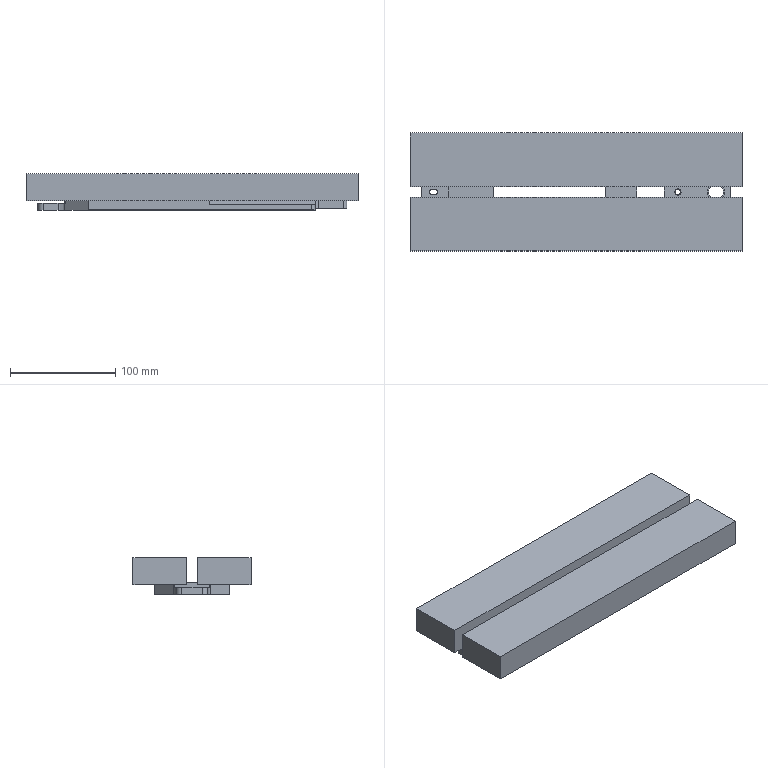NC program | NX | posted with a generic post | part box 315 x 112 x 34.85 mm
Lines 3199 to 4522 of 11462:
(ADAPTIVE_MILLING_COPY , TOOL : D4开粗)
N6390 T03 M6
N6392 G53
N6394 G17 G0 G90 X121.904 Y19.81 S6500 M3
N6396 G43 Z20. H3
N6398 Z-10.
N6400 G94 G1 X121.804 Y19.803 Z-10.625 F2000.
N6402 X121.705 Y19.797 Z-10.872
N6404 X121.605 Y19.79 Z-11.054
N6406 X121.505 Y19.783 Z-11.2
N6408 X121.405 Y19.776 Z-11.323
N6410 X121.306 Y19.769 Z-11.428
N6412 X121.206 Y19.762 Z-11.52
N6414 X121.106 Y19.755 Z-11.6
N6416 X121.006 Y19.748 Z-11.67
N6418 X120.907 Y19.741 Z-11.732
N6420 X120.807 Y19.734 Z-11.786
N6422 X120.707 Y19.727 Z-11.833
N6424 X120.607 Y19.72 Z-11.874
N6426 X120.507 Y19.713 Z-11.908
N6428 X120.408 Y19.706 Z-11.936
N6430 X120.308 Y19.699 Z-11.96
N6432 X120.208 Y19.692 Z-11.977
N6434 X120.108 Y19.685 Z-11.99
N6436 X120.009 Y19.678 Z-11.997
N6438 X119.909 Y19.671 Z-12.
N6440 X119.565 Y19.651
N6442 X119.222 Y19.614
N6444 G3 X118.932 Y19.226 R0.405
N6446 X119.957 Y16.307 R3.97
N6448 X122.288 Y14.7 R5.019
N6450 G1 X123.6
N6452 G2 X121.918 Y14.735 R12.158
N6454 X119.43 Y16.653 R4.439
N6456 X118.934 Y17.688 R3.914
N6458 G1 X118.933 Y18.626
N6460 G3 X118.965 Y17.166 R10.215
N6462 X121.068 Y14.709 R3.865
N6464 G1 X122.177 Y14.7
N6466 X120.959 Y14.713
N6468 G2 X119.174 Y16.174 R3.119
N6470 X118.936 Y16.705 R2.049
N6472 G1 X118.935 Y17.417
N6474 G3 X118.981 Y16.226 R5.673
N6476 X120.256 Y14.709 R2.419
N6478 G1 X121.068 Y14.7
N6480 G2 X120.115 Y14.725 R4.858
N6482 X118.937 Y15.953 R1.926
N6484 G1 X118.936 Y16.516
N6486 G3 X118.983 Y15.549 R3.764
N6488 X119.671 Y14.716 R1.364
N6490 G1 X120.245 Y14.7
N6492 G2 X119.567 Y14.73 R2.419
N6494 X118.937 Y15.773 R0.951
N6496 G3 X118.964 Y15.262 R4.171
N6498 X119.494 Y14.731 R1.08
N6500 G1 X119.676 Y14.702
N6502 G3 X120.106 Y15.099 R0.404
N6504 G1 X120.115 Y15.688
N6506 X120.116 Y15.788 Z-11.997
N6508 X120.118 Y15.888 Z-11.99
N6510 X120.119 Y15.988 Z-11.977
N6512 X120.121 Y16.088 Z-11.96
N6514 X120.122 Y16.188 Z-11.936
N6516 X120.124 Y16.288 Z-11.908
N6518 X120.126 Y16.388 Z-11.874
N6520 X120.127 Y16.488 Z-11.833
N6522 X120.129 Y16.588 Z-11.786
N6524 X120.13 Y16.688 Z-11.732
N6526 X120.132 Y16.788 Z-11.67
N6528 X120.133 Y16.888 Z-11.6
N6530 X120.135 Y16.988 Z-11.52
N6532 X120.136 Y17.088 Z-11.428
N6534 X120.138 Y17.188 Z-11.323
N6536 X120.139 Y17.288 Z-11.2
N6538 X120.141 Y17.388 Z-11.054
N6540 X120.142 Y17.488 Z-10.872
N6542 X120.144 Y17.588 Z-10.625
N6544 X120.145 Y17.688 Z-10.
N6546 G0 Z20.
N6548 X123.964 Y-17.678
N6550 Z-10.
N6552 G1 X123.962 Y-17.578 Z-10.625
N6554 X123.96 Y-17.478 Z-10.872
N6556 X123.959 Y-17.378 Z-11.054
N6558 X123.957 Y-17.278 Z-11.2
N6560 X123.955 Y-17.178 Z-11.323
N6562 X123.953 Y-17.078 Z-11.428
N6564 X123.952 Y-16.978 Z-11.52
N6566 X123.95 Y-16.878 Z-11.6
N6568 X123.948 Y-16.778 Z-11.67
N6570 X123.947 Y-16.678 Z-11.732
N6572 X123.945 Y-16.578 Z-11.786
N6574 X123.943 Y-16.478 Z-11.833
N6576 X123.941 Y-16.378 Z-11.874
N6578 X123.94 Y-16.278 Z-11.908
N6580 X123.938 Y-16.178 Z-11.936
N6582 X123.936 Y-16.078 Z-11.96
N6584 X123.935 Y-15.978 Z-11.977
N6586 X123.933 Y-15.878 Z-11.99
N6588 X123.931 Y-15.778 Z-11.997
N6590 X123.929 Y-15.678 Z-12.
N6592 X123.919 Y-15.097
N6594 G3 X123.515 Y-14.7 R0.404
N6596 X120.433 Y-15.812 R4.064
N6598 X118.911 Y-18.098 R5.039
N6600 G1 Y-19.336
N6602 G2 X118.947 Y-17.724 R11.256
N6604 X121.099 Y-15.067 R4.557
N6606 X121.932 Y-14.7 R3.985
N6608 G1 X122.832
N6610 G3 X121.442 Y-14.721 R15.425
N6612 X119.137 Y-16.454 R3.876
N6614 X118.911 Y-16.925 R1.387
N6616 G1 Y-18.013
N6618 X118.924 Y-16.757
N6620 G2 X120.344 Y-14.977 R3.165
N6622 X120.94 Y-14.7 R2.17
N6624 G1 X121.615
N6626 G3 X120.446 Y-14.749 R5.1
N6628 X118.928 Y-16.015 R2.666
N6630 G1 X118.911 Y-16.854
N6632 G2 X118.93 Y-15.934 R14.426
N6634 X120.192 Y-14.7 R1.931
N6636 G1 X120.717
N6638 G3 X119.73 Y-14.764 R3.043
N6640 X118.921 Y-15.476 R1.314
N6642 G1 X118.911 Y-16.03
N6644 G2 X118.958 Y-15.307 R2.219
N6646 X120.024 Y-14.7 R0.974
N6648 G3 X119.37 Y-14.781 R1.316
N6650 X118.927 Y-15.393 R1.202
N6652 X119.331 Y-15.862 R0.404
N6654 G1 X119.898 Y-15.854
N6656 X119.998 Y-15.853 Z-11.997
N6658 X120.098 Y-15.852 Z-11.99
N6660 X120.198 Y-15.851 Z-11.977
N6662 X120.298 Y-15.849 Z-11.96
N6664 X120.398 Y-15.848 Z-11.936
N6666 X120.498 Y-15.847 Z-11.908
N6668 X120.598 Y-15.845 Z-11.874
N6670 X120.698 Y-15.844 Z-11.833
N6672 X120.798 Y-15.843 Z-11.786
N6674 X120.898 Y-15.842 Z-11.732
N6676 X120.998 Y-15.84 Z-11.67
N6678 X121.098 Y-15.839 Z-11.6
N6680 X121.198 Y-15.838 Z-11.52
N6682 X121.298 Y-15.837 Z-11.428
N6684 X121.398 Y-15.835 Z-11.323
N6686 X121.498 Y-15.834 Z-11.2
N6688 X121.598 Y-15.833 Z-11.054
N6690 X121.698 Y-15.832 Z-10.872
N6692 X121.798 Y-15.83 Z-10.625
N6694 X121.898 Y-15.829 Z-10.
N6696 G0 Z20.
N6698 X134.278 Y0.889
N6700 Z2.
N6702 G3 X134.278 Y0.889 Z1.803 I-1.564 J-0.891
N6704 X134.278 Y0.889 Z1.605 I-1.564 J-0.891
N6706 X134.278 Y0.889 Z1.408 I-1.564 J-0.891
N6708 X134.278 Y0.889 Z1.21 I-1.564 J-0.891
N6710 X134.278 Y0.889 Z1.013 I-1.564 J-0.891
N6712 X134.278 Y0.889 Z0.816 I-1.564 J-0.891
N6714 X134.278 Y0.889 Z0.618 I-1.564 J-0.891
N6716 X134.278 Y0.889 Z0.421 I-1.564 J-0.891
N6718 X134.278 Y0.889 Z0.223 I-1.564 J-0.891
N6720 X134.278 Y0.889 Z0.026 I-1.564 J-0.891
N6722 X134.278 Y0.889 Z-0.172 I-1.564 J-0.891
N6724 X134.278 Y0.889 Z-0.369 I-1.564 J-0.891
N6726 X134.278 Y0.889 Z-0.566 I-1.564 J-0.891
N6728 X134.278 Y0.889 Z-0.764 I-1.564 J-0.891
N6730 X134.278 Y0.889 Z-0.961 I-1.564 J-0.891
N6732 X134.278 Y0.889 Z-1.159 I-1.564 J-0.891
N6734 X134.278 Y0.889 Z-1.356 I-1.564 J-0.891
N6736 X134.278 Y0.889 Z-1.553 I-1.564 J-0.891
N6738 X134.278 Y0.889 Z-1.751 I-1.564 J-0.891
N6740 X134.278 Y0.889 Z-1.948 I-1.564 J-0.891
N6742 X134.278 Y0.889 Z-2.146 I-1.564 J-0.891
N6744 X134.278 Y0.889 Z-2.343 I-1.564 J-0.891
N6746 X134.278 Y0.889 Z-2.54 I-1.564 J-0.891
N6748 X134.278 Y0.889 Z-2.738 I-1.564 J-0.891
N6750 X134.278 Y0.889 Z-2.935 I-1.564 J-0.891
N6752 X134.278 Y0.889 Z-3.133 I-1.564 J-0.891
N6754 X134.278 Y0.889 Z-3.33 I-1.564 J-0.891
N6756 X134.278 Y0.889 Z-3.528 I-1.564 J-0.891
N6758 X134.278 Y0.889 Z-3.725 I-1.564 J-0.891
N6760 X134.278 Y0.889 Z-3.922 I-1.564 J-0.891
N6762 X134.278 Y0.889 Z-4.12 I-1.564 J-0.891
N6764 X134.278 Y0.889 Z-4.317 I-1.564 J-0.891
N6766 X134.278 Y0.889 Z-4.515 I-1.564 J-0.891
N6768 X134.278 Y0.889 Z-4.712 I-1.564 J-0.891
N6770 X134.278 Y0.889 Z-4.909 I-1.564 J-0.891
N6772 X134.278 Y0.889 Z-5.107 I-1.564 J-0.891
N6774 X134.278 Y0.889 Z-5.304 I-1.564 J-0.891
N6776 X134.278 Y0.889 Z-5.502 I-1.564 J-0.891
N6778 X134.278 Y0.889 Z-5.699 I-1.564 J-0.891
N6780 X134.278 Y0.889 Z-5.896 I-1.564 J-0.891
N6782 X134.278 Y0.889 Z-6.094 I-1.564 J-0.891
N6784 X134.278 Y0.889 Z-6.291 I-1.564 J-0.891
N6786 X134.278 Y0.889 Z-6.489 I-1.564 J-0.891
N6788 X134.278 Y0.889 Z-6.686 I-1.564 J-0.891
N6790 X134.278 Y0.889 Z-6.884 I-1.564 J-0.891
N6792 X134.278 Y0.889 Z-7.081 I-1.564 J-0.891
N6794 X134.278 Y0.889 Z-7.278 I-1.564 J-0.891
N6796 X134.278 Y0.889 Z-7.476 I-1.564 J-0.891
N6798 X134.278 Y0.889 Z-7.673 I-1.564 J-0.891
N6800 X134.278 Y0.889 Z-7.871 I-1.564 J-0.891
N6802 X134.278 Y0.889 Z-8.068 I-1.564 J-0.891
N6804 X134.278 Y0.889 Z-8.265 I-1.564 J-0.891
N6806 X134.278 Y0.889 Z-8.463 I-1.564 J-0.891
N6808 X134.278 Y0.889 Z-8.66 I-1.564 J-0.891
N6810 X134.278 Y0.889 Z-8.858 I-1.564 J-0.891
N6812 X134.278 Y0.889 Z-9.055 I-1.564 J-0.891
N6814 X134.278 Y0.889 Z-9.252 I-1.564 J-0.891
N6816 X134.278 Y0.889 Z-9.45 I-1.564 J-0.891
N6818 X134.278 Y0.889 Z-9.647 I-1.564 J-0.891
N6820 X134.278 Y0.889 Z-9.845 I-1.564 J-0.891
N6822 X134.278 Y0.889 Z-10.042 I-1.564 J-0.891
N6824 X134.278 Y0.889 Z-10.24 I-1.564 J-0.891
N6826 X134.278 Y0.889 Z-10.437 I-1.564 J-0.891
N6828 X134.278 Y0.889 Z-10.634 I-1.564 J-0.891
N6830 X134.278 Y0.889 Z-10.832 I-1.564 J-0.891
N6832 X134.278 Y0.889 Z-11.029 I-1.564 J-0.891
N6834 X134.278 Y0.889 Z-11.227 I-1.564 J-0.891
N6836 X134.278 Y0.889 Z-11.424 I-1.564 J-0.891
N6838 X134.278 Y0.889 Z-11.621 I-1.564 J-0.891
N6840 X134.278 Y0.889 Z-11.819 I-1.564 J-0.891
N6842 X134.513 Y-0.002 Z-12. R-1.8
N6844 X133.169 Y-1.769 R-1.812
N6846 X134.378 Y1.134 R1.985
N6848 X131.316 Y-1.517 R-2.04
N6850 X134.785 Y-0.555 R2.149
N6852 X131.6 Y2.013 R2.19
N6854 X134.178 Y-1.829 R-2.321
N6856 X131.742 Y2.378 R2.448
N6858 X134.157 Y-2.179 R-2.59
N6860 X131.562 Y2.607 R2.728
N6862 X134.288 Y-2.437 R-2.875
N6864 X131.354 Y2.834 R3.02
N6866 X134.271 Y-2.792 R-3.17
N6868 X131.293 Y3.141 R3.321
N6870 X134.269 Y-3.141 R-3.476
N6872 X131.393 Y3.522 R3.632
N6874 X129.192 Y-1.367 R3.791
N6876 X134.1 Y-3.561 R3.791
N6878 X131.462 Y3.888 R3.952
N6880 X134.377 Y-3.804 R-4.117
N6882 X131.257 Y4.171 R4.284
N6884 X134.314 Y-4.192 R-4.452
N6886 X131.411 Y4.575 R4.621
N6888 X128.891 Y2.852 R4.753
N6890 X129.877 Y-3.871 R4.764
N6892 X132.631 Y-4.795 R5.129
N6894 X136.255 Y-3.234 R4.972
N6896 X135.347 Y4.007 R4.816
N6898 X133.403 Y4.748 R5.586
N6900 X130.734 Y4.369 R5.227
N6902 X129.688 Y3.725 R7.287
N6904 G1 X128.929 Y2.948
N6906 G3 X128.027 Y1.029 R5.459
N6908 X127.928 Y-0.178 R5.861
N6910 X128.347 Y-1.982 R4.669
N6912 X129.877 Y-3.871 R4.678
N6914 G1 X130.771 Y-4.383
N6916 G3 X131.297 Y-4.089 R0.404
N6918 G1 X131.415 Y-3.565
N6920 X131.437 Y-3.467 Z-11.997
N6922 X131.459 Y-3.37 Z-11.99
N6924 X131.481 Y-3.272 Z-11.977
N6926 X131.503 Y-3.175 Z-11.96
N6928 X131.525 Y-3.077 Z-11.936
N6930 X131.547 Y-2.98 Z-11.908
N6932 X131.569 Y-2.882 Z-11.874
N6934 X131.591 Y-2.785 Z-11.833
N6936 X131.613 Y-2.687 Z-11.786
N6938 X131.635 Y-2.59 Z-11.732
N6940 X131.657 Y-2.492 Z-11.67
N6942 X131.679 Y-2.394 Z-11.6
N6944 X131.701 Y-2.297 Z-11.52
N6946 X131.723 Y-2.199 Z-11.428
N6948 X131.745 Y-2.102 Z-11.323
N6950 X131.767 Y-2.004 Z-11.2
N6952 X131.789 Y-1.907 Z-11.054
N6954 X131.811 Y-1.809 Z-10.872
N6956 X131.833 Y-1.712 Z-10.625
N6958 X131.855 Y-1.614 Z-10.
N6960 G0 Z20.
N6962 X130.749 Y3.453
N6964 Z-1.
N6966 G1 X130.686 Y3.376 Z-1.625
N6968 X130.622 Y3.298 Z-1.872
N6970 X130.559 Y3.221 Z-2.054
N6972 X130.495 Y3.144 Z-2.2
N6974 X130.432 Y3.066 Z-2.323
N6976 X130.368 Y2.989 Z-2.428
N6978 X130.305 Y2.912 Z-2.52
N6980 X130.241 Y2.835 Z-2.6
N6982 X130.178 Y2.757 Z-2.67
N6984 X130.114 Y2.68 Z-2.732
N6986 X130.051 Y2.603 Z-2.786
N6988 X129.987 Y2.526 Z-2.833
N6990 X129.924 Y2.448 Z-2.874
N6992 X129.86 Y2.371 Z-2.908
N6994 X129.797 Y2.294 Z-2.936
N6996 X129.733 Y2.217 Z-2.96
N6998 X129.67 Y2.139 Z-2.977
N7000 X129.606 Y2.062 Z-2.99
N7002 X129.543 Y1.985 Z-2.997
N7004 X129.479 Y1.908 Z-3.
N7006 X127.934 Y0.016
N7008 G3 X127.828 Y-1.414 R2.078
N7010 X131.848 Y-5.074 R4.902
N7012 X127.68 Y1.115 R-5.151
N7014 X127.732 Y-2.277 R4.916
N7016 X135.519 Y-4.758 R5.442
N7018 X127.427 Y1.649 R-5.528
N7020 X127.808 Y-3.225 R5.441
N7022 X138.044 Y2.534 R5.885
N7024 X127.193 Y2.139 R5.921
N7026 X126.664 Y-0.024 R6.313
N7028 X127.104 Y-2.263 R6.904
N7030 X128.26 Y-4.094 R6.989
N7032 X130.91 Y-5.774 R6.428
N7034 X133.23 Y-6.024 R7.001
N7036 X134.632 Y-5.734 R9.787
N7038 X137.27 Y-3.971 R6.477
N7040 X138.699 Y-0.84 R6.338
N7042 X138.369 Y2.133 R6.079
N7044 X136.469 Y4.736 R6.48
N7046 X134.312 Y5.831 R6.722
N7048 G1 X133.152 Y6.03
N7050 G3 X130.788 Y5.735 R6.94
N7052 X128.122 Y3.939 R6.486
N7054 X126.755 Y1.049 R6.445
N7056 G1 X126.693 Y0.377
N7058 G3 X127.185 Y-0.054 R0.404
N7060 G1 X127.648 Y0.05
N7062 X127.745 Y0.072 Z-2.997
N7064 X127.843 Y0.095 Z-2.99
N7066 X127.94 Y0.117 Z-2.977
N7068 X128.038 Y0.139 Z-2.96
N7070 X128.135 Y0.161 Z-2.936
N7072 X128.233 Y0.183 Z-2.908
N7074 X128.33 Y0.205 Z-2.874
N7076 X128.428 Y0.227 Z-2.833
N7078 X128.525 Y0.249 Z-2.786
N7080 X128.623 Y0.271 Z-2.732
N7082 X128.721 Y0.293 Z-2.67
N7084 X128.818 Y0.315 Z-2.6
N7086 X128.916 Y0.337 Z-2.52
N7088 X129.013 Y0.359 Z-2.428
N7090 X129.111 Y0.381 Z-2.323
N7092 X129.208 Y0.403 Z-2.2
N7094 X129.306 Y0.425 Z-2.054
N7096 X129.403 Y0.448 Z-1.872
N7098 X129.501 Y0.47 Z-1.625
N7100 X129.598 Y0.492 Z-1.
N7102 G0 Z20.
N7104 X64.758 Y11.336
N7106 Z-3.399
N7108 G1 X64.745 Y11.435 Z-4.024
N7110 X64.732 Y11.535 Z-4.271
N7112 X64.719 Y11.634 Z-4.453
N7114 X64.706 Y11.733 Z-4.599
N7116 X64.693 Y11.832 Z-4.722
N7118 X64.68 Y11.931 Z-4.827
N7120 X64.667 Y12.03 Z-4.919
N7122 X64.653 Y12.13 Z-4.999
N7124 X64.64 Y12.229 Z-5.069
N7126 X64.627 Y12.328 Z-5.131
N7128 X64.614 Y12.427 Z-5.185
N7130 X64.601 Y12.526 Z-5.232
N7132 X64.588 Y12.625 Z-5.273
N7134 X64.575 Y12.724 Z-5.307
N7136 X64.562 Y12.824 Z-5.335
N7138 X64.549 Y12.923 Z-5.359
N7140 X64.536 Y13.022 Z-5.376
N7142 X64.523 Y13.121 Z-5.389
N7144 X64.51 Y13.22 Z-5.396
N7146 X64.497 Y13.319 Z-5.399
N7148 X64.414 Y13.949
N7150 G3 X64.014 Y14.3 R0.405
N7152 X61.361 Y13.372 R3.686
N7154 X59.763 Y11.186 R5.239
N7156 G1 X59.76 Y9.995
N7158 G2 X59.786 Y11.45 R11.987
N7160 X61.618 Y13.825 R4.291
N7162 X62.599 Y14.3 R3.662
N7164 G1 X63.461
N7166 G3 X62.042 Y14.259 R7.886
N7168 X59.771 Y12.298 R3.756
N7170 G1 X59.76 Y11.252
N7172 X59.777 Y12.422
N7174 G2 X61.652 Y14.3 R2.987
N7176 G1 X62.327
N7178 G3 X61.166 Y14.25 R4.906
N7180 X59.774 Y13.088 R2.354
N7182 G1 X59.76 Y12.298
N7184 G2 X59.78 Y13.179 R8.525
N7186 X60.935 Y14.3 R1.783
N7188 G1 X61.46
N7190 G3 X60.529 Y14.25 R3.228
N7192 X59.767 Y13.58 R1.152
N7194 G1 X59.76 Y13.08
N7196 G2 X59.82 Y13.787 R1.636
N7198 X60.755 Y14.3 R0.872
N7200 G3 X60.026 Y14.201 R1.328
N7202 X59.76 Y13.591 R0.57
N7204 G2 X60.04 Y14.251 R0.623
N7206 X60.319 Y14.3 R1.273
N7208 G3 X59.846 Y14.084 R0.503
N7210 X60.097 Y13.489 R0.404
N7212 G1 X60.766 Y13.322
N7214 X60.863 Y13.297 Z-5.396
N7216 X60.96 Y13.273 Z-5.389
N7218 X61.057 Y13.249 Z-5.376
N7220 X61.154 Y13.225 Z-5.359
N7222 X61.251 Y13.2 Z-5.335
N7224 X61.348 Y13.176 Z-5.307
N7226 X61.445 Y13.152 Z-5.273
N7228 X61.542 Y13.128 Z-5.232
N7230 X61.639 Y13.103 Z-5.185
N7232 X61.736 Y13.079 Z-5.131
N7234 X61.833 Y13.055 Z-5.069
N7236 X61.93 Y13.031 Z-4.999
N7238 X62.027 Y13.006 Z-4.919
N7240 X62.124 Y12.982 Z-4.827
N7242 X62.221 Y12.958 Z-4.722
N7244 X62.318 Y12.933 Z-4.599
N7246 X62.415 Y12.909 Z-4.453
N7248 X62.512 Y12.885 Z-4.271
N7250 X62.609 Y12.861 Z-4.024
N7252 X62.706 Y12.836 Z-3.399
N7254 G0 Z20.
N7256 X62.72 Y-9.246
N7258 Z-3.399
N7260 G1 X62.621 Y-9.259 Z-4.024
N7262 X62.522 Y-9.272 Z-4.271
N7264 X62.423 Y-9.286 Z-4.453
N7266 X62.324 Y-9.299 Z-4.599
N7268 X62.225 Y-9.312 Z-4.722
N7270 X62.125 Y-9.326 Z-4.827
N7272 X62.026 Y-9.339 Z-4.919
N7274 X61.927 Y-9.352 Z-4.999
N7276 X61.828 Y-9.365 Z-5.069
N7278 X61.729 Y-9.379 Z-5.131
N7280 X61.63 Y-9.392 Z-5.185
N7282 X61.531 Y-9.405 Z-5.232
N7284 X61.432 Y-9.419 Z-5.273
N7286 X61.333 Y-9.432 Z-5.307
N7288 X61.233 Y-9.445 Z-5.335
N7290 X61.134 Y-9.459 Z-5.359
N7292 X61.035 Y-9.472 Z-5.376
N7294 X60.936 Y-9.485 Z-5.389
N7296 X60.837 Y-9.499 Z-5.396
N7298 X60.738 Y-9.512 Z-5.399
N7300 X60.11 Y-9.596
N7302 G3 X59.76 Y-9.997 R0.405
N7304 X60.767 Y-12.784 R3.773
N7306 X62.914 Y-14.299 R5.114
N7308 G1 X64.091 Y-14.3
N7310 G2 X62.641 Y-14.275 R10.456
N7312 X60.207 Y-12.39 R4.325
N7314 X59.76 Y-11.446 R3.597
N7316 G1 Y-10.546
N7318 G3 X59.787 Y-11.944 R10.425
N7320 X61.779 Y-14.29 R3.71
N7322 G1 X62.82 Y-14.3
N7324 G2 X61.647 Y-14.282 R25.901
N7326 X59.765 Y-12.434 R3.082
N7328 G1 X59.76 Y-11.722
N7330 G3 X59.812 Y-12.891 R4.812
N7332 X60.992 Y-14.289 R2.313
N7334 G1 X61.779 Y-14.3
N7336 G2 X60.862 Y-14.274 R4.34
N7338 X59.76 Y-13.116 R1.795
N7340 G1 Y-12.591
N7342 G3 X59.806 Y-13.512 R3.43
N7344 X60.465 Y-14.289 R1.205
N7346 G1 X61.027 Y-14.3
N7348 G2 X60.339 Y-14.27 R2.257
N7350 X59.76 Y-13.269 R0.902
N7352 G3 X59.823 Y-13.966 R1.564
N7354 X60.469 Y-14.3 R0.571
N7356 G2 X59.809 Y-14.02 R0.623
N7358 X59.76 Y-13.741 R1.273
N7360 G3 X59.976 Y-14.214 R0.503
N7362 X60.571 Y-13.962 R0.404
N7364 G1 X60.738 Y-13.293
N7366 X60.762 Y-13.196 Z-5.396
N7368 X60.786 Y-13.099 Z-5.389
N7370 X60.81 Y-13.002 Z-5.376
N7372 X60.835 Y-12.905 Z-5.359
N7374 X60.859 Y-12.808 Z-5.335
N7376 X60.883 Y-12.711 Z-5.307
N7378 X60.907 Y-12.614 Z-5.273
N7380 X60.931 Y-12.517 Z-5.232
N7382 X60.956 Y-12.42 Z-5.185
N7384 X60.98 Y-12.323 Z-5.131
N7386 X61.004 Y-12.226 Z-5.069
N7388 X61.028 Y-12.129 Z-4.999
N7390 X61.052 Y-12.032 Z-4.919
N7392 X61.077 Y-11.934 Z-4.827
N7394 X61.101 Y-11.837 Z-4.722
N7396 X61.125 Y-11.74 Z-4.599
N7398 X61.149 Y-11.643 Z-4.453
N7400 X61.173 Y-11.546 Z-4.271
N7402 X61.197 Y-11.449 Z-4.024
N7404 X61.222 Y-11.352 Z-3.399
N7406 G0 Z20.
N7408 X76.611 Y-11.341
N7410 Z-3.399
N7412 G1 X76.625 Y-11.44 Z-4.024
N7414 X76.639 Y-11.539 Z-4.271
N7416 X76.652 Y-11.638 Z-4.453
N7418 X76.666 Y-11.737 Z-4.599
N7420 X76.679 Y-11.836 Z-4.722
N7422 X76.693 Y-11.935 Z-4.827
N7424 X76.706 Y-12.034 Z-4.919
N7426 X76.72 Y-12.133 Z-4.999
N7428 X76.734 Y-12.232 Z-5.069
N7430 X76.747 Y-12.331 Z-5.131
N7432 X76.761 Y-12.43 Z-5.185
N7434 X76.774 Y-12.53 Z-5.232
N7436 X76.788 Y-12.629 Z-5.273
N7438 X76.802 Y-12.728 Z-5.307
N7440 X76.815 Y-12.827 Z-5.335
N7442 X76.829 Y-12.926 Z-5.359
N7444 X76.842 Y-13.025 Z-5.376
N7446 X76.856 Y-13.124 Z-5.389
N7448 X76.869 Y-13.223 Z-5.396
N7450 X76.883 Y-13.322 Z-5.399
N7452 X76.969 Y-13.951
N7454 G3 X77.369 Y-14.3 R0.405
N7456 X80.057 Y-13.367 R3.73
N7458 X81.656 Y-11.187 R5.33
N7460 G1 X81.66 Y-9.987
N7462 G2 X81.633 Y-11.446 R11.629
N7464 X79.787 Y-13.83 R4.305
N7466 X78.809 Y-14.3 R3.67
N7468 G1 X77.909
N7470 G3 X79.309 Y-14.272 R9.962
N7472 X81.65 Y-12.291 R3.711
N7474 G1 X81.66 Y-11.248
N7476 G2 X81.641 Y-12.422 R21.265
N7478 X79.781 Y-14.298 R3.062
N7480 G1 X79.083 Y-14.3
N7482 G3 X80.193 Y-14.265 R5.498
N7484 X81.644 Y-13.089 R2.4
N7486 G1 X81.66 Y-12.292
N7488 X81.643 Y-13.167
N7490 G2 X80.475 Y-14.3 R1.77
N7492 G1 X79.95
N7494 G3 X80.917 Y-14.24 R3.008
N7496 X81.648 Y-13.597 R1.194
N7498 G1 X81.66 Y-13.073
N7500 G2 X81.628 Y-13.727 R1.949
N7502 X80.634 Y-14.3 R0.896
N7504 G3 X81.319 Y-14.241 R1.614
N7506 X81.66 Y-13.591 R0.573
N7508 G2 X81.38 Y-14.251 R0.623
N7510 X81.101 Y-14.3 R1.273
N7512 G3 X81.574 Y-14.084 R0.503
N7514 X81.323 Y-13.489 R0.404
N7516 G1 X80.656 Y-13.322
N7518 X80.559 Y-13.298 Z-5.396
N7520 X80.462 Y-13.273 Z-5.389
N7522 X80.365 Y-13.249 Z-5.376
N7524 X80.268 Y-13.225 Z-5.359
N7526 X80.171 Y-13.201 Z-5.335
N7528 X80.074 Y-13.176 Z-5.307
N7530 X79.977 Y-13.152 Z-5.273
N7532 X79.88 Y-13.128 Z-5.232
N7534 X79.783 Y-13.103 Z-5.185
N7536 X79.686 Y-13.079 Z-5.131
N7538 X79.589 Y-13.055 Z-5.069
N7540 X79.492 Y-13.03 Z-4.999
N7542 X79.395 Y-13.006 Z-4.919
N7544 X79.298 Y-12.982 Z-4.827
N7546 X79.201 Y-12.958 Z-4.722
N7548 X79.104 Y-12.933 Z-4.599
N7550 X79.007 Y-12.909 Z-4.453
N7552 X78.91 Y-12.885 Z-4.271
N7554 X78.813 Y-12.86 Z-4.024
N7556 X78.716 Y-12.836 Z-3.399
N7558 G0 Z20.
N7560 X78.701 Y9.224
N7562 Z-3.399
N7564 G1 X78.8 Y9.237 Z-4.024
N7566 X78.899 Y9.251 Z-4.271
N7568 X78.998 Y9.264 Z-4.453
N7570 X79.097 Y9.278 Z-4.599
N7572 X79.196 Y9.292 Z-4.722
N7574 X79.295 Y9.305 Z-4.827
N7576 X79.394 Y9.319 Z-4.919
N7578 X79.493 Y9.332 Z-4.999
N7580 X79.592 Y9.346 Z-5.069
N7582 X79.691 Y9.36 Z-5.131
N7584 X79.79 Y9.373 Z-5.185
N7586 X79.89 Y9.387 Z-5.232
N7588 X79.989 Y9.401 Z-5.273
N7590 X80.088 Y9.414 Z-5.307
N7592 X80.187 Y9.428 Z-5.335
N7594 X80.286 Y9.441 Z-5.359
N7596 X80.385 Y9.455 Z-5.376
N7598 X80.484 Y9.469 Z-5.389
N7600 X80.583 Y9.482 Z-5.396
N7602 X80.682 Y9.496 Z-5.399
N7604 X81.311 Y9.582
N7606 G3 X81.66 Y9.983 R0.405
N7608 X80.706 Y12.715 R3.771
N7610 X78.575 Y14.295 R5.546
N7612 G1 X77.411 Y14.3
N7614 G2 X78.791 Y14.276 R11.555
N7616 X81.113 Y12.532 R4.259
N7618 X81.66 Y11.435 R3.646
N7620 G1 Y10.573
N7622 G3 X81.619 Y11.998 R8.101
N7624 X79.664 Y14.286 R3.795
N7626 G1 X78.609 Y14.3
N7628 X79.754 Y14.285
N7630 G2 X81.657 Y12.415 R3.033
N7632 G1 X81.66 Y11.714
N7634 G3 X81.61 Y12.881 R4.938
N7636 X80.421 Y14.29 R2.283
N7638 G1 X79.641 Y14.3
N7640 G2 X80.556 Y14.275 R4.432
N7642 X81.66 Y13.114 R1.807
N7644 G1 Y12.589
N7646 G3 X81.611 Y13.521 R3.343
N7648 X80.959 Y14.287 R1.22
N7650 G1 X80.397 Y14.3
N7652 G2 X81.132 Y14.245 R1.848
N7654 X81.66 Y13.301 R0.882
N7656 G3 X81.534 Y14.076 R1.267
N7658 X80.951 Y14.3 R0.554
N7660 G2 X81.611 Y14.02 R0.623
N7662 X81.66 Y13.741 R1.273
N7664 G3 X81.444 Y14.214 R0.503
N7666 X80.849 Y13.963 R0.404
N7668 G1 X80.682 Y13.295
N7670 X80.658 Y13.198 Z-5.396
N7672 X80.634 Y13.101 Z-5.389
N7674 X80.609 Y13.004 Z-5.376
N7676 X80.585 Y12.907 Z-5.359
N7678 X80.561 Y12.81 Z-5.335
N7680 X80.537 Y12.713 Z-5.307
N7682 X80.512 Y12.616 Z-5.273
N7684 X80.488 Y12.519 Z-5.232
N7686 X80.464 Y12.422 Z-5.185
N7688 X80.44 Y12.325 Z-5.131
N7690 X80.415 Y12.228 Z-5.069
N7692 X80.391 Y12.131 Z-4.999
N7694 X80.367 Y12.034 Z-4.919
N7696 X80.342 Y11.937 Z-4.827
N7698 X80.318 Y11.84 Z-4.722
N7700 X80.294 Y11.743 Z-4.599
N7702 X80.27 Y11.646 Z-4.453
N7704 X80.245 Y11.549 Z-4.271
N7706 X80.221 Y11.452 Z-4.024
N7708 X80.197 Y11.355 Z-3.399
N7710 G0 Z20.
N7712 X-124.018 Y-20.986
N7714 Z-1.
N7716 G1 X-123.945 Y-20.917 Z-1.625
N7718 X-123.872 Y-20.849 Z-1.872
N7720 X-123.799 Y-20.781 Z-2.054
N7722 X-123.726 Y-20.712 Z-2.2
N7724 X-123.653 Y-20.644 Z-2.323
N7726 X-123.58 Y-20.576 Z-2.428
N7728 X-123.507 Y-20.507 Z-2.52
N7730 X-123.434 Y-20.439 Z-2.6
N7732 X-123.361 Y-20.371 Z-2.67
N7734 X-123.288 Y-20.302 Z-2.732
N7736 X-123.215 Y-20.234 Z-2.786
N7738 X-123.142 Y-20.165 Z-2.833
N7740 X-123.069 Y-20.097 Z-2.874
N7742 X-122.996 Y-20.029 Z-2.908
N7744 X-122.923 Y-19.96 Z-2.936
N7746 X-122.851 Y-19.892 Z-2.96
N7748 X-122.778 Y-19.824 Z-2.977
N7750 X-122.705 Y-19.755 Z-2.99
N7752 X-122.632 Y-19.687 Z-2.997
N7754 X-122.559 Y-19.619 Z-3.
N7756 X-122.083 Y-19.173
N7758 G3 X-122.014 Y-18.669 R0.405
N7760 G1 X-122.307 Y-18.186
N7762 G2 X-122.7 Y-16.262 R4.855
N7764 G3 X-123.11 Y-15.858 R0.404
N7766 G1 X-123.678 Y-15.865
N7768 X-123.778 Y-15.867 Z-2.997
N7770 X-123.878 Y-15.868 Z-2.99
N7772 X-123.978 Y-15.869 Z-2.977
N7774 X-124.078 Y-15.871 Z-2.96
N7776 X-124.178 Y-15.872 Z-2.936
N7778 X-124.278 Y-15.874 Z-2.908
N7780 X-124.378 Y-15.875 Z-2.874
N7782 X-124.478 Y-15.876 Z-2.833
N7784 X-124.578 Y-15.878 Z-2.786
N7786 X-124.678 Y-15.879 Z-2.732
N7788 X-124.778 Y-15.88 Z-2.67
N7790 X-124.878 Y-15.882 Z-2.6
N7792 X-124.978 Y-15.883 Z-2.52
N7794 X-125.078 Y-15.884 Z-2.428
N7796 X-125.178 Y-15.886 Z-2.323
N7798 X-125.278 Y-15.887 Z-2.2
N7800 X-125.378 Y-15.889 Z-2.054
N7802 X-125.478 Y-15.89 Z-1.872
N7804 X-125.578 Y-15.891 Z-1.625
N7806 X-125.678 Y-15.893 Z-1.
N7808 G0 Z20.
N7810 Y16.233
N7812 Z-1.
N7814 G1 X-125.578 Z-1.625
N7816 X-125.478 Y16.232 Z-1.872
N7818 X-125.378 Z-2.054
N7820 X-125.278 Y16.231 Z-2.2
N7822 X-125.178 Z-2.323
N7824 X-125.078 Z-2.428
N7826 X-124.978 Y16.23 Z-2.52
N7828 X-124.878 Z-2.6
N7830 X-124.778 Z-2.67
N7832 X-124.678 Y16.229 Z-2.732
N7834 X-124.578 Z-2.786
N7836 X-124.478 Z-2.833
N7838 X-124.378 Y16.228 Z-2.874
N7840 X-124.278 Z-2.908
N7842 X-124.178 Z-2.936
N7844 X-124.078 Y16.227 Z-2.96
N7846 X-123.978 Z-2.977
N7848 X-123.878 Y16.226 Z-2.99
N7850 X-123.778 Z-2.997
N7852 X-123.678 Z-3.
N7854 X-123.339 Y16.221
N7856 X-123. Y16.232
N7858 G3 X-122.681 Y16.584 R0.405
N7860 G1 X-122.601 Y17.32
N7862 X-122.307 Y18.186
N7864 X-122.054 Y18.602
N7866 G3 X-122.129 Y19.112 R0.405
N7868 G1 X-122.612 Y19.549
N7870 X-122.686 Y19.616 Z-2.997
N7872 X-122.761 Y19.683 Z-2.99
N7874 X-122.835 Y19.75 Z-2.977
N7876 X-122.909 Y19.817 Z-2.96
N7878 X-122.983 Y19.884 Z-2.936
N7880 X-123.057 Y19.951 Z-2.908
N7882 X-123.132 Y20.018 Z-2.874
N7884 X-123.206 Y20.085 Z-2.833
N7886 X-123.28 Y20.152 Z-2.786
N7888 X-123.354 Y20.219 Z-2.732
N7890 X-123.428 Y20.286 Z-2.67
N7892 X-123.503 Y20.353 Z-2.6
N7894 X-123.577 Y20.42 Z-2.52
N7896 X-123.651 Y20.487 Z-2.428
N7898 X-123.725 Y20.554 Z-2.323
N7900 X-123.799 Y20.621 Z-2.2
N7902 X-123.874 Y20.688 Z-2.054
N7904 X-123.948 Y20.755 Z-1.872
N7906 X-124.022 Y20.822 Z-1.625
N7908 X-124.096 Y20.889 Z-1.
N7910 G0 Z20.
N7912 X18.806 Y40.862
N7914 Z-2.
N7916 G1 X18.774 Y40.767 Z-2.625
N7918 X18.743 Y40.672 Z-2.872
N7920 X18.712 Y40.577 Z-3.054
N7922 X18.68 Y40.482 Z-3.2
N7924 X18.649 Y40.387 Z-3.323
N7926 X18.618 Y40.292 Z-3.428
N7928 X18.587 Y40.198 Z-3.52
N7930 X18.555 Y40.103 Z-3.6
N7932 X18.524 Y40.008 Z-3.67
N7934 X18.493 Y39.913 Z-3.732
N7936 X18.461 Y39.818 Z-3.786
N7938 X18.43 Y39.723 Z-3.833
N7940 X18.399 Y39.628 Z-3.874
N7942 X18.368 Y39.533 Z-3.908
N7944 X18.336 Y39.438 Z-3.936
N7946 X18.305 Y39.343 Z-3.96
N7948 X18.274 Y39.248 Z-3.977
N7950 X18.242 Y39.153 Z-3.99
N7952 X18.211 Y39.058 Z-3.997
N7954 X18.18 Y38.963 Z-4.
N7956 X18.082 Y38.674
N7958 X17.998 Y38.382
N7960 G3 X18.328 Y37.942 R0.404
N7962 G1 X20.652 Y37.519
N7964 G3 X21.109 Y37.793 R0.405
N7966 G1 X21.304 Y38.395
N7968 X21.334 Y38.49 Z-3.997
N7970 X21.365 Y38.585 Z-3.99
N7972 X21.396 Y38.68 Z-3.977
N7974 X21.427 Y38.775 Z-3.96
N7976 X21.457 Y38.871 Z-3.936
N7978 X21.488 Y38.966 Z-3.908
N7980 X21.519 Y39.061 Z-3.874
N7982 X21.55 Y39.156 Z-3.833
N7984 X21.58 Y39.251 Z-3.786
N7986 X21.611 Y39.346 Z-3.732
N7988 X21.642 Y39.441 Z-3.67
N7990 X21.673 Y39.537 Z-3.6
N7992 X21.703 Y39.632 Z-3.52
N7994 X21.734 Y39.727 Z-3.428
N7996 X21.765 Y39.822 Z-3.323
N7998 X21.796 Y39.917 Z-3.2
N8000 X21.827 Y40.012 Z-3.054
N8002 X21.857 Y40.108 Z-2.872
N8004 X21.888 Y40.203 Z-2.625
N8006 X21.919 Y40.298 Z-2.
N8008 G0 Z20.
N8010 X72.273 Y0.889
N8012 Z2.
N8014 G3 X72.273 Y0.889 Z1.803 I-1.564 J-0.891
N8016 X72.273 Y0.889 Z1.605 I-1.564 J-0.891
N8018 X72.273 Y0.889 Z1.408 I-1.564 J-0.891
N8020 X72.273 Y0.889 Z1.21 I-1.564 J-0.891
N8022 X72.273 Y0.889 Z1.013 I-1.564 J-0.891
N8024 X72.273 Y0.889 Z0.816 I-1.564 J-0.891
N8026 X72.273 Y0.889 Z0.618 I-1.564 J-0.891
N8028 X72.273 Y0.889 Z0.421 I-1.564 J-0.891
N8030 X72.273 Y0.889 Z0.223 I-1.564 J-0.891
N8032 X72.273 Y0.889 Z0.026 I-1.564 J-0.891
N8034 X72.273 Y0.889 Z-0.172 I-1.564 J-0.891
N8036 X72.273 Y0.889 Z-0.369 I-1.564 J-0.891
N8038 X72.273 Y0.889 Z-0.566 I-1.564 J-0.891
N8040 X72.273 Y0.889 Z-0.764 I-1.564 J-0.891
N8042 X72.273 Y0.889 Z-0.961 I-1.564 J-0.891
N8044 X72.273 Y0.889 Z-1.159 I-1.564 J-0.891
N8046 X72.273 Y0.889 Z-1.356 I-1.564 J-0.891
N8048 X72.273 Y0.889 Z-1.553 I-1.564 J-0.891
N8050 X72.273 Y0.889 Z-1.751 I-1.564 J-0.891
N8052 X72.273 Y0.889 Z-1.948 I-1.564 J-0.891
N8054 X72.273 Y0.889 Z-2.146 I-1.564 J-0.891
N8056 X72.273 Y0.889 Z-2.343 I-1.564 J-0.891
N8058 X72.273 Y0.889 Z-2.54 I-1.564 J-0.891
N8060 X72.273 Y0.889 Z-2.738 I-1.564 J-0.891
N8062 X72.273 Y0.889 Z-2.935 I-1.564 J-0.891
N8064 X72.273 Y0.889 Z-3.133 I-1.564 J-0.891
N8066 X72.273 Y0.889 Z-3.33 I-1.564 J-0.891
N8068 X72.273 Y0.889 Z-3.528 I-1.564 J-0.891
N8070 X72.273 Y0.889 Z-3.725 I-1.564 J-0.891
N8072 X72.273 Y0.889 Z-3.922 I-1.564 J-0.891
N8074 X72.273 Y0.889 Z-4.12 I-1.564 J-0.891
N8076 X72.273 Y0.889 Z-4.317 I-1.564 J-0.891
N8078 X72.273 Y0.889 Z-4.515 I-1.564 J-0.891
N8080 X72.273 Y0.889 Z-4.712 I-1.564 J-0.891
N8082 X72.273 Y0.889 Z-4.909 I-1.564 J-0.891
N8084 X72.273 Y0.889 Z-5.107 I-1.564 J-0.891
N8086 X72.273 Y0.889 Z-5.304 I-1.564 J-0.891
N8088 X72.273 Y0.889 Z-5.502 I-1.564 J-0.891
N8090 X72.273 Y0.889 Z-5.699 I-1.564 J-0.891
N8092 X72.273 Y0.889 Z-5.896 I-1.564 J-0.891
N8094 X72.273 Y0.889 Z-6.094 I-1.564 J-0.891
N8096 X72.273 Y0.889 Z-6.291 I-1.564 J-0.891
N8098 X72.273 Y0.889 Z-6.489 I-1.564 J-0.891
N8100 X72.273 Y0.889 Z-6.686 I-1.564 J-0.891
N8102 X72.273 Y0.889 Z-6.884 I-1.564 J-0.891
N8104 X72.273 Y0.889 Z-7.081 I-1.564 J-0.891
N8106 X72.273 Y0.889 Z-7.278 I-1.564 J-0.891
N8108 X72.273 Y0.889 Z-7.476 I-1.564 J-0.891
N8110 X72.273 Y0.889 Z-7.673 I-1.564 J-0.891
N8112 X72.273 Y0.889 Z-7.871 I-1.564 J-0.891
N8114 X72.273 Y0.889 Z-8.068 I-1.564 J-0.891
N8116 X72.273 Y0.889 Z-8.265 I-1.564 J-0.891
N8118 X72.273 Y0.889 Z-8.463 I-1.564 J-0.891
N8120 X72.273 Y0.889 Z-8.66 I-1.564 J-0.891
N8122 X72.273 Y0.889 Z-8.858 I-1.564 J-0.891
N8124 X72.273 Y0.889 Z-9.055 I-1.564 J-0.891
N8126 X72.273 Y0.889 Z-9.252 I-1.564 J-0.891
N8128 X72.273 Y0.889 Z-9.45 I-1.564 J-0.891
N8130 X72.273 Y0.889 Z-9.647 I-1.564 J-0.891
N8132 X72.273 Y0.889 Z-9.845 I-1.564 J-0.891
N8134 X72.273 Y0.889 Z-10.042 I-1.564 J-0.891
N8136 X72.273 Y0.889 Z-10.24 I-1.564 J-0.891
N8138 X72.273 Y0.889 Z-10.437 I-1.564 J-0.891
N8140 X72.273 Y0.889 Z-10.634 I-1.564 J-0.891
N8142 X72.273 Y0.889 Z-10.832 I-1.564 J-0.891
N8144 X72.273 Y0.889 Z-11.029 I-1.564 J-0.891
N8146 X72.273 Y0.889 Z-11.227 I-1.564 J-0.891
N8148 X72.273 Y0.889 Z-11.424 I-1.564 J-0.891
N8150 X72.273 Y0.889 Z-11.621 I-1.564 J-0.891
N8152 X72.273 Y0.889 Z-11.819 I-1.564 J-0.891
N8154 X72.508 Y-0.002 Z-12. R-1.8
N8156 X71.164 Y-1.769 R-1.812
N8158 X72.373 Y1.134 R1.985
N8160 X69.432 Y-1.619 R-2.04
N8162 X72.828 Y-0.4 R2.158
N8164 X69.452 Y1.928 R2.197
N8166 X72.172 Y-1.828 R-2.321
N8168 X69.738 Y2.378 R2.447
N8170 X72.151 Y-2.177 R-2.59
N8172 X69.557 Y2.609 R2.728
N8174 X72.282 Y-2.437 R-2.875
N8176 X69.35 Y2.836 R3.021
N8178 X72.264 Y-2.793 R-3.17
N8180 X69.291 Y3.145 R3.321
N8182 X72.442 Y-3.049 R-3.478
N8184 X69.595 Y3.595 R3.632
N8186 X72.286 Y-3.48 R-3.791
N8188 X69.893 Y4.002 R3.949
N8190 X72.156 Y-3.885 R-4.114
N8192 X74.895 Y0.97 R4.241
N8194 X71.682 Y4.3 R4.244
N8196 X69.735 Y4.266 R17.09
N8198 X66.397 Y-1.127 R4.332
N8200 X69.511 Y-4.3 R4.452
N8202 X71.795 Y-4.273 R26.132
N8204 X75.305 Y-0.431 R4.368
N8206 X72.751 Y4.285 R4.611
N8208 G1 X71.656 Y4.3
N8210 G2 X72.926 Y4.268 R7.473
N8212 X74.91 Y2.534 R3.643
N8214 X72.53 Y-4.289 R4.738
N8216 G1 X71.518 Y-4.3
N8218 G3 X73.001 Y-4.267 R9.651
N8220 X75.177 Y-2.511 R3.744
N8222 X74.05 Y4.056 R5.032
N8224 X73.582 Y4.3 R1.119
N8226 G1 X72.72
N8228 G2 X73.785 Y4.277 R7.436
N8230 X75.314 Y2.955 R3.084
N8232 X74.327 Y-3.802 R5.182
N8234 X73.429 Y-4.3 R2.423
N8236 G1 X72.791
N8238 G3 X73.923 Y-4.249 R4.668
N8240 X75.768 Y-2.617 R3.495
N8242 X75.061 Y3.838 R5.418
N8244 X74.37 Y4.3 R1.419
N8246 G1 X73.62
N8248 G2 X74.573 Y4.274 R4.649
N8250 X75.962 Y2.979 R2.913
N8252 X75.273 Y-3.61 R5.532
N8254 X74.22 Y-4.3 R2.377
N8256 G1 X73.62
N8258 G3 X74.686 Y-4.245 R3.958
N8260 X76.364 Y-2.704 R3.295
N8262 X75.923 Y3.658 R5.737
N8264 X75.147 Y4.292 R1.91
N8266 G1 X74.417 Y4.3
N8268 G2 X75.284 Y4.277 R5.398
N8270 X76.584 Y3.032 R2.747
N8272 X76.093 Y-3.459 R5.817
N8274 X74.95 Y-4.299 R2.458
N8276 G1 X74.376 Y-4.3
N8278 G3 X75.401 Y-4.241 R3.469
N8280 X77.02 Y-2.677 R3.244
N8282 X76.66 Y3.571 R5.969
N8284 X75.853 Y4.288 R2.04
N8286 G1 X75.141 Y4.3
N8288 G2 X75.981 Y4.273 R3.38
N8290 X77.23 Y3.034 R2.684
N8292 X76.794 Y-3.405 R6.017
N8294 X75.644 Y-4.298 R2.476
N8296 G1 X75.096 Y-4.3
N8298 G3 X76.07 Y-4.242 R3.224
N8300 X77.631 Y-2.718 R3.163
N8302 X77.374 Y3.489 R6.15
N8304 X76.537 Y4.283 R2.25
N8306 G1 X75.848 Y4.3
N8308 G2 X76.614 Y4.281 R8.253
N8310 X77.806 Y3.147 R2.458
N8312 X77.481 Y-3.348 R6.158
N8314 X76.344 Y-4.291 R2.779
N8316 G1 X75.796 Y-4.3
N8318 G3 X76.74 Y-4.237 R2.868
N8320 X78.292 Y-2.663 R3.182
N8322 X78.054 Y3.438 R6.277
N8324 X77.178 Y4.287 R2.156
N8326 G1 X76.503 Y4.3
N8328 X77.262 Y4.283
N8330 G2 X78.425 Y3.181 R2.387
N8332 X78.161 Y-3.29 R6.273
N8334 X76.964 Y-4.296 R2.548
N8336 G1 X76.439 Y-4.3
N8338 G3 X77.382 Y-4.237 R2.871
N8340 X78.911 Y-2.684 R3.138
N8342 X78.734 Y3.375 R6.379
N8344 X77.836 Y4.283 R2.297
N8346 G1 X77.147 Y4.3
N8348 G2 X77.946 Y4.272 R3.156
N8350 X79.154 Y3.015 R2.6
N8352 X78.814 Y-3.263 R6.374
N8354 X77.62 Y-4.293 R2.684
N8356 G1 X77.086 Y-4.3
N8358 G3 X78.04 Y-4.23 R2.69
N8360 X79.529 Y-2.701 R3.143
N8362 X79.369 Y3.377 R6.425
N8364 X78.474 Y4.285 R2.225
N8366 G1 X77.791 Y4.3
N8368 G2 X78.56 Y4.279 R5.367
N8370 X79.735 Y3.111 R2.43
N8372 X79.442 Y-3.264 R6.405
N8374 X78.254 Y-4.293 R2.643
N8376 G1 X77.759 Y-4.3
N8378 G3 X78.649 Y-4.239 R2.547
N8380 X80.135 Y-2.742 R3.081
N8382 X80.022 Y3.346 R6.472
N8384 X79.146 Y4.273 R2.627
N8386 X78.463 Y4.3 R2.788
N8388 G2 X79.192 Y4.28 R6.361
N8390 X80.361 Y3.122 R2.405
N8392 X80.091 Y-3.234 R6.447
N8394 X78.916 Y-4.287 R2.851
N8396 G1 X78.392 Y-4.3
N8398 G3 X79.324 Y-4.22 R2.474
N8400 X80.815 Y-2.638 R3.202
N8402 X80.693 Y3.282 R6.533
N8404 X79.781 Y4.273 R2.685
N8406 X79.097 Y4.3 R2.732
N8408 G2 X79.857 Y4.272 R3.083
N8410 X81.058 Y3.001 R2.574
N8412 X81.653 Y-0.3 R6.527
N8414 X80.305 Y-3.743 R5.457
N8416 X79.466 Y-4.3 R1.759
N8418 G1 X78.978
N8420 G3 X79.933 Y-4.229 R2.676
N8422 X81.439 Y-2.641 R3.166
N8424 X81.66 Y-2.08 R4.116
N8426 G1 Y-0.13
N8428 G2 X81.641 Y-2.363 R37.013
N8430 X80.161 Y-4.287 R2.765
N8432 G1 X79.636 Y-4.3
N8434 G3 X80.578 Y-4.212 R2.338
N8436 X81.654 Y-3.115 R2.065
N8438 G1 X81.66 Y-2.173
N8440 X81.646 Y-3.232
N8442 G2 X80.678 Y-4.294 R1.633
N8444 G1 X80.222 Y-4.3
N8446 G3 X81.02 Y-4.245 R2.287
N8448 X81.66 Y-3.443 R0.901
N8450 G1 Y-3.143
N8452 G2 X81.471 Y-3.982 R1.175
N8454 X80.84 Y-4.295 R0.848
N8456 X80.424 Y-4.063 R0.401
N8458 G1 X80.162 Y-3.326 Z-11.9
N8460 X80.105 Y-3.175 F15000.
N8462 X80.07 Y-3.018
N8464 X80.326 Y0.024
N8466 G2 X80.662 Y0.385 R0.401
N8468 G1 X81.323 Y0.399 Z-11.985 F2000.
N8470 X81.438 Y0.436 Z-12.
N8472 G3 X81.66 Y0.794 R0.402
N8474 X81.603 Y2.375 R8.495
N8476 X80.433 Y4.257 R3.046
N8478 X79.712 Y4.3 R2.19
N8480 G2 X80.444 Y4.279 R5.238
N8482 X81.578 Y3.042 R2.219
N8484 G1 X81.66 Y2.793
N8486 Y1.931
N8488 G3 X81.627 Y3.257 R8.241
N8490 X80.878 Y4.283 R1.496
N8492 G1 X80.336 Y4.3
N8494 G2 X81.038 Y4.24 R1.751
N8496 X81.66 Y3.443 R1.114
N8498 G1 Y3.031
N8500 G3 X81.54 Y3.892 R1.739
N8502 X80.931 Y4.281 R0.822
N8504 X80.461 Y4.017 R0.403
N8506 G1 X80.324 Y3.691 Z-11.955
N8508 X80.175 Y3.37 Z-11.909
N8510 X80.129 Y3.312 Z-11.9
N8512 G2 X79.842 Y3.192 R0.408 F15000.
N8514 G1 X71.121 Y3.211
N8516 G2 X70.872 Y3.299 R0.415
N8518 G1 X70.765 Y3.427 Z-11.921 F2000.
N8520 X70.682 Y3.573 Z-11.943
N8522 X70.459 Y3.96 Z-12.
N8524 G3 X70.258 Y4.23 R0.757
N8526 X70.032 Y4.3 R2.175
N8528 X68.733 Y4.21 R4.386
N8530 X66.089 Y1.324 R4.209
N8532 X68.531 Y-4.29 R4.759
N8534 G1 X69.534 Y-4.3
N8536 G2 X68.391 Y-4.281 R17.453
N8538 X66.552 Y-2.82 R3.503
N8540 X67.753 Y3.961 R4.865
N8542 X68.474 Y4.3 R2.379
N8544 G1 X69.224
N8546 G3 X67.992 Y4.264 R6.898
N8548 X66.035 Y2.614 R3.475
N8550 X67.329 Y-4.128 R5.147
N8552 X67.699 Y-4.3 R0.901
N8554 G1 X68.524
N8556 G2 X67.497 Y-4.278 R8.365
N8558 X65.967 Y-2.966 R3.098
N8560 X66.555 Y3.616 R5.29
N8562 X67.628 Y4.3 R2.39
N8564 G1 X68.228
N8566 G3 X67.145 Y4.247 R4.128
N8568 X65.387 Y2.605 R3.374
N8570 X66.243 Y-3.867 R5.521
N8572 X66.905 Y-4.3 R1.376
N8574 G1 X67.655
N8576 X66.742 Y-4.284
N8578 G2 X65.391 Y-3.114 R2.731
N8580 X65.755 Y3.499 R5.613
N8582 X66.861 Y4.298 R2.52
N8584 G1 X67.407 Y4.3
N8586 G3 X66.416 Y4.24 R3.332
N8588 X64.781 Y2.659 R3.244
N8590 X65.373 Y-3.689 R5.818
N8592 X66.134 Y-4.293 R1.826
N8594 G1 X66.854 Y-4.3
N8596 G2 X66.013 Y-4.282 R13.479
N8598 X64.717 Y-3.097 R2.639
N8600 X64.977 Y3.352 R5.885
N8602 X66.174 Y4.298 R2.527
N8604 G1 X66.721 Y4.3
N8606 G3 X65.745 Y4.242 R3.256
N8608 X64.189 Y2.727 R3.135
N8610 X64.634 Y-3.612 R6.018
N8612 X65.405 Y-4.285 R2.15
N8614 G1 X66.124 Y-4.3
N8616 X65.329 Y-4.284
N8618 G2 X64.092 Y-3.144 R2.518
N8620 X64.295 Y3.295 R6.066
N8622 X65.474 Y4.291 R2.776
N8624 G1 X66.019 Y4.3
N8626 G3 X65.057 Y4.23 R2.765
N8628 X63.521 Y2.651 R3.192
N8630 X63.875 Y-3.478 R6.207
N8632 X64.732 Y-4.285 R2.235
N8634 G1 X65.413 Y-4.3
N8636 G2 X64.646 Y-4.28 R6.695
N8638 X63.438 Y-3.134 R2.495
N8640 X63.642 Y3.268 R6.202
N8642 X64.85 Y4.296 R2.559
N8644 G1 X65.375 Y4.3
N8646 G3 X64.419 Y4.231 R2.762
N8648 X62.892 Y2.642 R3.169
N8650 X63.221 Y-3.471 R6.3
N8652 X64.069 Y-4.284 R2.227
N8654 G1 X64.755 Y-4.3
N8656 G2 X63.994 Y-4.282 R19.831
N8658 X62.816 Y-3.168 R2.423
N8660 X62.994 Y3.241 R6.297
N8662 X64.197 Y4.293 R2.691
N8664 G1 X64.733 Y4.3
N8666 G3 X63.787 Y4.232 R2.73
N8668 X62.297 Y2.698 R3.121
N8670 X62.55 Y-3.431 R6.375
N8672 X63.415 Y-4.283 R2.272
N8674 G1 X64.106 Y-4.3
N8676 G2 X63.306 Y-4.272 R3.171
N8678 X62.079 Y-2.994 R2.638
N8680 X62.334 Y3.189 R6.397
N8682 X63.563 Y4.293 R2.705
N8684 G1 X64.062 Y4.3
N8686 G3 X63.131 Y4.221 R2.483
N8688 X61.639 Y2.632 R3.18
N8690 X61.869 Y-3.367 R6.455
N8692 X62.772 Y-4.284 R2.282
N8694 G1 X63.458 Y-4.3
N8696 G2 X62.694 Y-4.281 R8.331
N8698 X61.533 Y-3.157 R2.404
N8700 X61.726 Y3.217 R6.417
N8702 X62.952 Y4.295 R2.584
N8704 G1 X63.476 Y4.3
N8706 G3 X62.531 Y4.233 R2.751
N8708 X61.046 Y2.692 R3.104
N8710 X61.213 Y-3.337 R6.493
N8712 X62.119 Y-4.28 R2.433
N8714 X62.787 Y-4.3 R7.612
N8716 G2 X62.023 Y-4.273 R3.043
N8718 X60.818 Y-3.013 R2.583
N8720 X61.121 Y3.245 R6.451
N8722 X62.304 Y4.291 R2.69
N8724 G1 X62.811 Y4.3
N8726 G3 X61.906 Y4.233 R2.573
N8728 X60.441 Y2.728 R3.088
N8730 X60.599 Y-3.37 R6.493
N8732 X61.482 Y-4.28 R2.357
N8734 X62.184 Y-4.3 R8.983
N8736 G2 X61.385 Y-4.273 R3.242
N8738 X60.186 Y-3.016 R2.568
N8740 X59.76 Y-1.876 R5.766
N8742 X59.781 Y1.337 R65.582
N8744 X61.348 Y4.123 R4.106
N8746 X61.738 Y4.3 R1.119
N8748 G1 X62.188
N8750 G3 X61.28 Y4.232 R2.551
N8752 X59.76 Y2.487 R2.91
N8754 G1 Y1.062
N8756 X59.773 Y2.687
N8758 G2 X61.081 Y4.292 R2.314
N8760 G1 X61.585 Y4.3
N8762 G3 X60.649 Y4.211 R2.256
N8764 X59.767 Y3.332 R1.631
N8766 G1 X59.76 Y2.537
N8768 G2 X59.779 Y3.452 R11.936
N8770 X60.617 Y4.3 R1.267
N8772 G1 X60.992
N8774 G3 X60.168 Y4.18 R1.683
N8776 X59.76 Y3.331 R0.908
N8778 G1 X59.774 Y-2.505
N8780 G3 X60.852 Y-4.269 R2.545
N8782 X61.546 Y-4.3 R2.393
N8784 G2 X60.779 Y-4.269 R2.962
N8786 X59.76 Y-3.039 R1.965
N8788 G1 Y-2.326
N8790 G3 X59.799 Y-3.472 R5.519
N8792 X60.372 Y-4.25 R1.211
N8794 X60.917 Y-4.3 R1.91
N8796 G2 X59.872 Y-3.864 R1.06
N8798 X59.76 Y-3.256 R1.413
N8800 G3 X59.857 Y-3.836 R1.367
N8802 X60.308 Y-4.232 R0.753
N8804 X60.816 Y-3.862 R0.404
N8806 G1 X60.843 Y-3.308
N8808 X60.848 Y-3.208 Z-11.997
N8810 X60.853 Y-3.108 Z-11.99
N8812 X60.858 Y-3.008 Z-11.977
N8814 X60.863 Y-2.908 Z-11.96
N8816 X60.868 Y-2.808 Z-11.936
N8818 X60.873 Y-2.708 Z-11.908
N8820 X60.878 Y-2.608 Z-11.874
N8822 X60.883 Y-2.509 Z-11.833
N8824 X60.888 Y-2.409 Z-11.786
N8826 X60.893 Y-2.309 Z-11.732
N8828 X60.898 Y-2.209 Z-11.67
N8830 X60.902 Y-2.109 Z-11.6
N8832 X60.907 Y-2.009 Z-11.52
N8834 X60.912 Y-1.909 Z-11.428
N8836 X60.917 Y-1.809 Z-11.323
N8838 X60.922 Y-1.71 Z-11.2
N8840 X60.927 Y-1.61 Z-11.054
N8842 X60.932 Y-1.51 Z-10.872
N8844 X60.937 Y-1.41 Z-10.625
N8846 X60.942 Y-1.31 Z-10.
N8848 G0 Z20.
N8850 M5
(DRILLING , TOOL : D8点钻)
N8852 T04 M6
N8854 G53
N8856 G17 G0 G90 X122.71 Y8.5 S2500 M3
N8858 G43 Z20. H4
N8860 G94 G81 G99 Z-1.7 F200. R3.
N8862 X142.71
N8864 Y-8.5
N8866 X122.71
N8868 G80
N8870 G0 X122.71 Y-8.5 Z20.
(DRILLING_COPY , TOOL : D8点钻)
N8872 X99.9 Y18.
N8874 G81 Z-2.6 F200. R3.
N8876 X93.52 Y-18.
N8878 G80
N8880 G0 X93.52 Y-18. Z20.
(DRILLING_COPY_COPY_1 , TOOL : D8点钻)
N8882 X96.71 Y0.
N8884 G81 Z-2.8 F200. R3.
N8886 G80
N8888 G0 X96.71 Y0. Z20.
(DRILLING_COPY_COPY , TOOL : D8点钻)
N8890 X13.21 Y30.
N8892 G81 Z-1.2 F200. R3.
N8894 X-72.29
N8896 Y-30.
N8898 X13.21
N8900 G80
N8902 G0 X13.21 Y-30. Z20.
N8904 M5
(DRILLING_COPY_1 , TOOL : D3.4_DRILL)
N8906 T05 M6
N8908 G53
N8910 G17 G0 G90 X122.71 Y8.5 S2500 M3
N8912 G43 Z20. H5
N8914 G94 G83 G99 Z-13. F200. Q2. R3.
N8916 X142.71
N8918 Y-8.5
N8920 X122.71
N8922 G80
N8924 G0 X122.71 Y-8.5 Z20.
N8926 M5
(DRILLING_COPY_COPY_2 , TOOL : D4.5_DRILL)
N8928 T06 M6
N8930 G53
N8932 G17 G0 G90 X96.71 Y0. S2500 M3
N8934 G43 Z20. H6
N8936 G94 G83 G99 Z-13. F200. Q2. R3.
N8938 X99.9 Y18.
N8940 G80
N8942 G0 X99.9 Y18. Z20.
N8944 M5
(DRILLING_COPY_COPY_2_COPY , TOOL : 5.5_DRILL)
N8946 T13 M6
N8948 G53
N8950 G17 G0 G90 X93.52 Y-18. S2500 M3
N8952 G43 Z20. H13
N8954 G94 G83 G99 Z-13. F200. Q2. R3.
N8956 G80
N8958 G0 X93.52 Y-18. Z20.
N8960 M5
(DRILLING_COPY_COPY_COPY , TOOL : D2.3_DRILL)
N8962 T07 M6
N8964 G53
N8966 G17 G0 G90 X13.21 Y30. S2500 M3
N8968 G43 Z20. H7
N8970 G94 G83 G99 Z-13. F200. Q2. R3.
N8972 X-72.29
N8974 Y-30.
N8976 X13.21
N8978 G80
N8980 G0 X13.21 Y-30. Z20.
N8982 M5